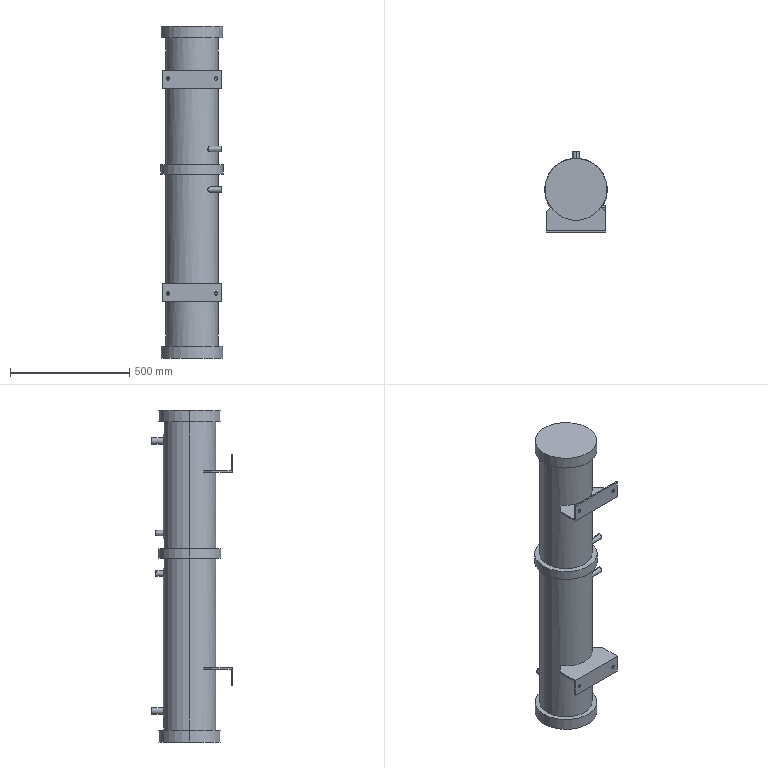Part | STEP file | 10+13RT condenser | 3 solids | 96 faces | box 263 x 339 x 1390 mm | volume 54968408 mm3 | cylinder 56 | plane 40 | commonest cylinder face diameters 219 x10 14 x8 19 x8 22 x8 6.35 x4 25 x4